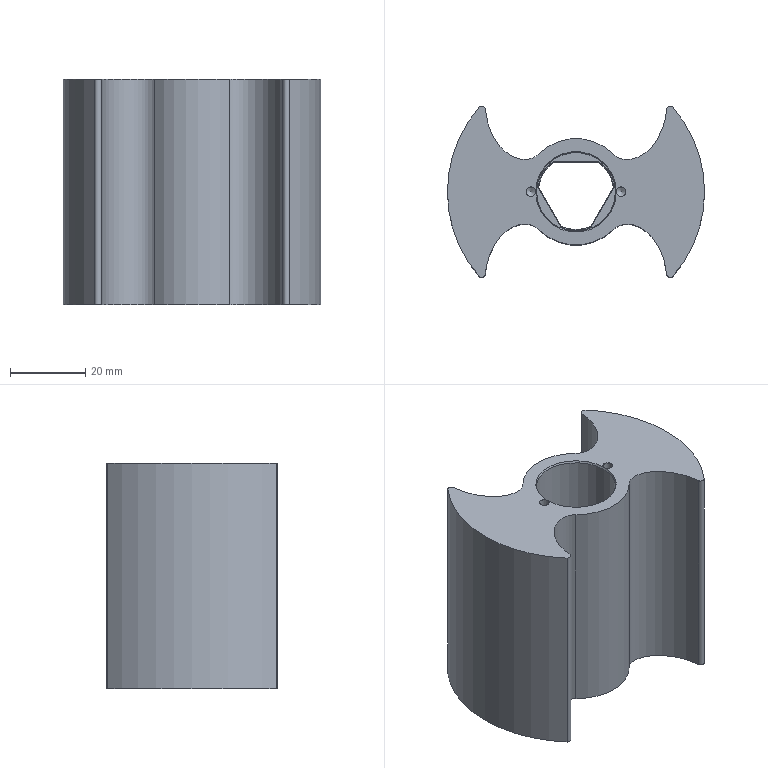NC program | NX | posted with a generic post | part box 68.489 x 45.577 x 60 mm
Lines 1 to 915 of 7016:
N10 G17 G21 G94 G90
(ZLEVEL_PROFILE_COPY_2 , TOOL : D25R0.5)
N12 T05 M6
N14 G54
N16 G17 G0 G90 X47.764 Y-35.886 S2000 M3
N18 G43 Z30. H5
N20 Z-0.349
N22 G94 G1 X43.686 Y-35.094 F1000.
N24 G3 X41.323 Y-35.908 R2.5
N26 G2 X7.37 Y-33.859 R21.45 F2200.
N28 G1 X7.248 Y-33.886
N30 G2 X-7.37 Y-33.859 R34.651
N32 X-41.323 Y-35.908 R21.45
N34 G3 X-43.686 Y-35.094 R2.5
N36 G1 X-47.764 Y-35.886
N38 G0 Z30.
N40 X47.766
N42 Z-0.698
N44 G1 X43.687 Y-35.094 F1000.
N46 G3 X41.323 Y-35.908 R2.5
N48 G2 X7.367 Y-33.86 R21.45 F2200.
N50 G1 X7.248 Y-33.889
N52 G2 X-7.248 Y-33.889 R34.655
N54 G1 X-7.367 Y-33.86
N56 G2 X-41.323 Y-35.908 R21.45
N58 G3 X-43.687 Y-35.094 R2.5
N60 G1 X-47.766 Y-35.886
N62 G0 Z30.
N64 X47.766
N66 Z-1.047
N68 G1 X43.687 Y-35.094 F1000.
N70 G3 X41.323 Y-35.908 R2.5
N72 G2 X7.367 Y-33.86 R21.45 F2200.
N74 G1 X7.248 Y-33.889
N76 G2 X-7.248 Y-33.889 R34.655
N78 G1 X-7.367 Y-33.86
N80 G2 X-41.323 Y-35.908 R21.45
N82 G3 X-43.687 Y-35.094 R2.5
N84 G1 X-47.766 Y-35.886
N86 G0 Z30.
N88 X47.766
N90 Z-1.395
N92 G1 X43.687 Y-35.094 F1000.
N94 G3 X41.323 Y-35.908 R2.5
N96 G2 X7.367 Y-33.86 R21.45 F2200.
N98 G1 X7.248 Y-33.889
N100 G2 X-7.248 Y-33.889 R34.655
N102 G1 X-7.367 Y-33.86
N104 G2 X-41.323 Y-35.908 R21.45
N106 G3 X-43.687 Y-35.094 R2.5
N108 G1 X-47.766 Y-35.886
N110 G0 Z30.
N112 X47.766
N114 Z-1.744
N116 G1 X43.687 Y-35.094 F1000.
N118 G3 X41.323 Y-35.908 R2.5
N120 G2 X7.367 Y-33.86 R21.45 F2200.
N122 G1 X7.248 Y-33.889
N124 G2 X-7.248 Y-33.889 R34.655
N126 G1 X-7.367 Y-33.86
N128 G2 X-41.323 Y-35.908 R21.45
N130 G3 X-43.687 Y-35.094 R2.5
N132 G1 X-47.766 Y-35.886
N134 G0 Z30.
N136 X47.766
N138 Z-2.093
N140 G1 X43.687 Y-35.094 F1000.
N142 G3 X41.323 Y-35.908 R2.5
N144 G2 X7.367 Y-33.86 R21.45 F2200.
N146 G1 X7.248 Y-33.889
N148 G2 X-7.248 Y-33.889 R34.655
N150 G1 X-7.367 Y-33.86
N152 G2 X-41.323 Y-35.908 R21.45
N154 G3 X-43.687 Y-35.094 R2.5
N156 G1 X-47.766 Y-35.886
N158 G0 Z30.
N160 X47.766
N162 Z-2.442
N164 G1 X43.687 Y-35.094 F1000.
N166 G3 X41.323 Y-35.908 R2.5
N168 G2 X7.367 Y-33.86 R21.45 F2200.
N170 G1 X7.248 Y-33.889
N172 G2 X-7.248 Y-33.889 R34.655
N174 G1 X-7.367 Y-33.86
N176 G2 X-41.323 Y-35.908 R21.45
N178 G3 X-43.687 Y-35.094 R2.5
N180 G1 X-47.766 Y-35.886
N182 G0 Z30.
N184 X47.766
N186 Z-2.791
N188 G1 X43.687 Y-35.094 F1000.
N190 G3 X41.323 Y-35.908 R2.5
N192 G2 X7.367 Y-33.86 R21.45 F2200.
N194 G1 X7.248 Y-33.889
N196 G2 X-7.248 Y-33.889 R34.655
N198 G1 X-7.367 Y-33.86
N200 G2 X-41.323 Y-35.908 R21.45
N202 G3 X-43.687 Y-35.094 R2.5
N204 G1 X-47.766 Y-35.886
N206 G0 Z30.
N208 X47.766
N210 Z-3.14
N212 G1 X43.687 Y-35.094 F1000.
N214 G3 X41.323 Y-35.908 R2.5
N216 G2 X7.367 Y-33.86 R21.45 F2200.
N218 G1 X7.248 Y-33.889
N220 G2 X-7.248 Y-33.889 R34.655
N222 G1 X-7.367 Y-33.86
N224 G2 X-41.323 Y-35.908 R21.45
N226 G3 X-43.687 Y-35.094 R2.5
N228 G1 X-47.766 Y-35.886
N230 G0 Z30.
N232 X47.766
N234 Z-3.488
N236 G1 X43.687 Y-35.094 F1000.
N238 G3 X41.323 Y-35.908 R2.5
N240 G2 X7.367 Y-33.86 R21.45 F2200.
N242 G1 X7.248 Y-33.889
N244 G2 X-7.248 Y-33.889 R34.655
N246 G1 X-7.367 Y-33.86
N248 G2 X-41.323 Y-35.908 R21.45
N250 G3 X-43.687 Y-35.094 R2.5
N252 G1 X-47.766 Y-35.886
N254 G0 Z30.
N256 X47.766
N258 Z-3.837
N260 G1 X43.687 Y-35.094 F1000.
N262 G3 X41.323 Y-35.908 R2.5
N264 G2 X7.367 Y-33.86 R21.45 F2200.
N266 G1 X7.248 Y-33.889
N268 G2 X-7.248 Y-33.889 R34.655
N270 G1 X-7.367 Y-33.86
N272 G2 X-41.323 Y-35.908 R21.45
N274 G3 X-43.687 Y-35.094 R2.5
N276 G1 X-47.766 Y-35.886
N278 G0 Z30.
N280 X47.766
N282 Z-4.186
N284 G1 X43.687 Y-35.094 F1000.
N286 G3 X41.323 Y-35.908 R2.5
N288 G2 X7.367 Y-33.86 R21.45 F2200.
N290 G1 X7.248 Y-33.889
N292 G2 X-7.248 Y-33.889 R34.655
N294 G1 X-7.367 Y-33.86
N296 G2 X-41.323 Y-35.908 R21.45
N298 G3 X-43.687 Y-35.094 R2.5
N300 G1 X-47.766 Y-35.886
N302 G0 Z30.
N304 X47.766
N306 Z-4.535
N308 G1 X43.687 Y-35.094 F1000.
N310 G3 X41.323 Y-35.908 R2.5
N312 G2 X7.367 Y-33.86 R21.45 F2200.
N314 G1 X7.248 Y-33.889
N316 G2 X-7.248 Y-33.889 R34.655
N318 G1 X-7.367 Y-33.86
N320 G2 X-41.323 Y-35.908 R21.45
N322 G3 X-43.687 Y-35.094 R2.5
N324 G1 X-47.766 Y-35.886
N326 G0 Z30.
N328 X47.766
N330 Z-4.884
N332 G1 X43.687 Y-35.094 F1000.
N334 G3 X41.323 Y-35.908 R2.5
N336 G2 X7.367 Y-33.86 R21.45 F2200.
N338 G1 X7.248 Y-33.889
N340 G2 X-7.248 Y-33.889 R34.655
N342 G1 X-7.367 Y-33.86
N344 G2 X-41.323 Y-35.908 R21.45
N346 G3 X-43.687 Y-35.094 R2.5
N348 G1 X-47.766 Y-35.886
N350 G0 Z30.
N352 X47.766
N354 Z-5.233
N356 G1 X43.687 Y-35.094 F1000.
N358 G3 X41.323 Y-35.908 R2.5
N360 G2 X7.367 Y-33.86 R21.45 F2200.
N362 G1 X7.248 Y-33.889
N364 G2 X-7.248 Y-33.889 R34.655
N366 G1 X-7.367 Y-33.86
N368 G2 X-41.323 Y-35.908 R21.45
N370 G3 X-43.687 Y-35.094 R2.5
N372 G1 X-47.766 Y-35.886
N374 G0 Z30.
N376 X47.766
N378 Z-5.581
N380 G1 X43.687 Y-35.094 F1000.
N382 G3 X41.323 Y-35.908 R2.5
N384 G2 X7.367 Y-33.86 R21.45 F2200.
N386 G1 X7.248 Y-33.889
N388 G2 X-7.248 Y-33.889 R34.655
N390 G1 X-7.367 Y-33.86
N392 G2 X-41.323 Y-35.908 R21.45
N394 G3 X-43.687 Y-35.094 R2.5
N396 G1 X-47.766 Y-35.886
N398 G0 Z30.
N400 X47.766
N402 Z-5.93
N404 G1 X43.687 Y-35.094 F1000.
N406 G3 X41.323 Y-35.908 R2.5
N408 G2 X7.367 Y-33.86 R21.45 F2200.
N410 G1 X7.248 Y-33.889
N412 G2 X-7.248 Y-33.889 R34.655
N414 G1 X-7.367 Y-33.86
N416 G2 X-41.323 Y-35.908 R21.45
N418 G3 X-43.687 Y-35.094 R2.5
N420 G1 X-47.766 Y-35.886
N422 G0 Z30.
N424 X47.766
N426 Z-6.279
N428 G1 X43.687 Y-35.094 F1000.
N430 G3 X41.323 Y-35.908 R2.5
N432 G2 X7.367 Y-33.86 R21.45 F2200.
N434 G1 X7.248 Y-33.889
N436 G2 X-7.248 Y-33.889 R34.655
N438 G1 X-7.367 Y-33.86
N440 G2 X-41.323 Y-35.908 R21.45
N442 G3 X-43.687 Y-35.094 R2.5
N444 G1 X-47.766 Y-35.886
N446 G0 Z30.
N448 X47.766
N450 Z-6.628
N452 G1 X43.687 Y-35.094 F1000.
N454 G3 X41.323 Y-35.908 R2.5
N456 G2 X7.367 Y-33.86 R21.45 F2200.
N458 G1 X7.248 Y-33.889
N460 G2 X-7.248 Y-33.889 R34.655
N462 G1 X-7.367 Y-33.86
N464 G2 X-41.323 Y-35.908 R21.45
N466 G3 X-43.687 Y-35.094 R2.5
N468 G1 X-47.766 Y-35.886
N470 G0 Z30.
N472 X47.766
N474 Z-6.977
N476 G1 X43.687 Y-35.094 F1000.
N478 G3 X41.323 Y-35.908 R2.5
N480 G2 X7.367 Y-33.86 R21.45 F2200.
N482 G1 X7.248 Y-33.889
N484 G2 X-7.248 Y-33.889 R34.655
N486 G1 X-7.367 Y-33.86
N488 G2 X-41.323 Y-35.908 R21.45
N490 G3 X-43.687 Y-35.094 R2.5
N492 G1 X-47.766 Y-35.886
N494 G0 Z30.
N496 X47.766
N498 Z-7.326
N500 G1 X43.687 Y-35.094 F1000.
N502 G3 X41.323 Y-35.908 R2.5
N504 G2 X7.367 Y-33.86 R21.45 F2200.
N506 G1 X7.248 Y-33.889
N508 G2 X-7.248 Y-33.889 R34.655
N510 G1 X-7.367 Y-33.86
N512 G2 X-41.323 Y-35.908 R21.45
N514 G3 X-43.687 Y-35.094 R2.5
N516 G1 X-47.766 Y-35.886
N518 G0 Z30.
N520 X47.766
N522 Z-7.674
N524 G1 X43.687 Y-35.094 F1000.
N526 G3 X41.323 Y-35.908 R2.5
N528 G2 X7.367 Y-33.86 R21.45 F2200.
N530 G1 X7.248 Y-33.889
N532 G2 X-7.248 Y-33.889 R34.655
N534 G1 X-7.367 Y-33.86
N536 G2 X-41.323 Y-35.908 R21.45
N538 G3 X-43.687 Y-35.094 R2.5
N540 G1 X-47.766 Y-35.886
N542 G0 Z30.
N544 X47.766
N546 Z-8.023
N548 G1 X43.687 Y-35.094 F1000.
N550 G3 X41.323 Y-35.908 R2.5
N552 G2 X7.367 Y-33.86 R21.45 F2200.
N554 G1 X7.248 Y-33.889
N556 G2 X-7.248 Y-33.889 R34.655
N558 G1 X-7.367 Y-33.86
N560 G2 X-41.323 Y-35.908 R21.45
N562 G3 X-43.687 Y-35.094 R2.5
N564 G1 X-47.766 Y-35.886
N566 G0 Z30.
N568 X47.766
N570 Z-8.372
N572 G1 X43.687 Y-35.094 F1000.
N574 G3 X41.323 Y-35.908 R2.5
N576 G2 X7.367 Y-33.86 R21.45 F2200.
N578 G1 X7.248 Y-33.889
N580 G2 X-7.248 Y-33.889 R34.655
N582 G1 X-7.367 Y-33.86
N584 G2 X-41.323 Y-35.908 R21.45
N586 G3 X-43.687 Y-35.094 R2.5
N588 G1 X-47.766 Y-35.886
N590 G0 Z30.
N592 X47.766
N594 Z-8.721
N596 G1 X43.687 Y-35.094 F1000.
N598 G3 X41.323 Y-35.908 R2.5
N600 G2 X7.367 Y-33.86 R21.45 F2200.
N602 G1 X7.248 Y-33.889
N604 G2 X-7.248 Y-33.889 R34.655
N606 G1 X-7.367 Y-33.86
N608 G2 X-41.323 Y-35.908 R21.45
N610 G3 X-43.687 Y-35.094 R2.5
N612 G1 X-47.766 Y-35.886
N614 G0 Z30.
N616 X47.766
N618 Z-9.07
N620 G1 X43.687 Y-35.094 F1000.
N622 G3 X41.323 Y-35.908 R2.5
N624 G2 X7.367 Y-33.86 R21.45 F2200.
N626 G1 X7.248 Y-33.889
N628 G2 X-7.248 Y-33.889 R34.655
N630 G1 X-7.367 Y-33.86
N632 G2 X-41.323 Y-35.908 R21.45
N634 G3 X-43.687 Y-35.094 R2.5
N636 G1 X-47.766 Y-35.886
N638 G0 Z30.
N640 X47.766
N642 Z-9.419
N644 G1 X43.687 Y-35.094 F1000.
N646 G3 X41.323 Y-35.908 R2.5
N648 G2 X7.367 Y-33.86 R21.45 F2200.
N650 G1 X7.248 Y-33.889
N652 G2 X-7.248 Y-33.889 R34.655
N654 G1 X-7.367 Y-33.86
N656 G2 X-41.323 Y-35.908 R21.45
N658 G3 X-43.687 Y-35.094 R2.5
N660 G1 X-47.766 Y-35.886
N662 G0 Z30.
N664 X47.766
N666 Z-9.767
N668 G1 X43.687 Y-35.094 F1000.
N670 G3 X41.323 Y-35.908 R2.5
N672 G2 X7.367 Y-33.86 R21.45 F2200.
N674 G1 X7.248 Y-33.889
N676 G2 X-7.248 Y-33.889 R34.655
N678 G1 X-7.367 Y-33.86
N680 G2 X-41.323 Y-35.908 R21.45
N682 G3 X-43.687 Y-35.094 R2.5
N684 G1 X-47.766 Y-35.886
N686 G0 Z30.
N688 X47.766
N690 Z-10.116
N692 G1 X43.687 Y-35.094 F1000.
N694 G3 X41.323 Y-35.908 R2.5
N696 G2 X7.367 Y-33.86 R21.45 F2200.
N698 G1 X7.248 Y-33.889
N700 G2 X-7.248 Y-33.889 R34.655
N702 G1 X-7.367 Y-33.86
N704 G2 X-41.323 Y-35.908 R21.45
N706 G3 X-43.687 Y-35.094 R2.5
N708 G1 X-47.766 Y-35.886
N710 G0 Z30.
N712 X47.766
N714 Z-10.465
N716 G1 X43.687 Y-35.094 F1000.
N718 G3 X41.323 Y-35.908 R2.5
N720 G2 X7.367 Y-33.86 R21.45 F2200.
N722 G1 X7.248 Y-33.889
N724 G2 X-7.248 Y-33.889 R34.655
N726 G1 X-7.367 Y-33.86
N728 G2 X-41.323 Y-35.908 R21.45
N730 G3 X-43.687 Y-35.094 R2.5
N732 G1 X-47.766 Y-35.886
N734 G0 Z30.
N736 X47.766
N738 Z-10.814
N740 G1 X43.687 Y-35.094 F1000.
N742 G3 X41.323 Y-35.908 R2.5
N744 G2 X7.367 Y-33.86 R21.45 F2200.
N746 G1 X7.248 Y-33.889
N748 G2 X-7.248 Y-33.889 R34.655
N750 G1 X-7.367 Y-33.86
N752 G2 X-41.323 Y-35.908 R21.45
N754 G3 X-43.687 Y-35.094 R2.5
N756 G1 X-47.766 Y-35.886
N758 G0 Z30.
N760 X47.766
N762 Z-11.163
N764 G1 X43.687 Y-35.094 F1000.
N766 G3 X41.323 Y-35.908 R2.5
N768 G2 X7.367 Y-33.86 R21.45 F2200.
N770 G1 X7.248 Y-33.889
N772 G2 X-7.248 Y-33.889 R34.655
N774 G1 X-7.367 Y-33.86
N776 G2 X-41.323 Y-35.908 R21.45
N778 G3 X-43.687 Y-35.094 R2.5
N780 G1 X-47.766 Y-35.886
N782 G0 Z30.
N784 X47.766
N786 Z-11.512
N788 G1 X43.687 Y-35.094 F1000.
N790 G3 X41.323 Y-35.908 R2.5
N792 G2 X7.367 Y-33.86 R21.45 F2200.
N794 G1 X7.248 Y-33.889
N796 G2 X-7.248 Y-33.889 R34.655
N798 G1 X-7.367 Y-33.86
N800 G2 X-41.323 Y-35.908 R21.45
N802 G3 X-43.687 Y-35.094 R2.5
N804 G1 X-47.766 Y-35.886
N806 G0 Z30.
N808 X47.766
N810 Z-11.86
N812 G1 X43.687 Y-35.094 F1000.
N814 G3 X41.323 Y-35.908 R2.5
N816 G2 X7.367 Y-33.86 R21.45 F2200.
N818 G1 X7.248 Y-33.889
N820 G2 X-7.248 Y-33.889 R34.655
N822 G1 X-7.367 Y-33.86
N824 G2 X-41.323 Y-35.908 R21.45
N826 G3 X-43.687 Y-35.094 R2.5
N828 G1 X-47.766 Y-35.886
N830 G0 Z30.
N832 X47.766
N834 Z-12.209
N836 G1 X43.687 Y-35.094 F1000.
N838 G3 X41.323 Y-35.908 R2.5
N840 G2 X7.367 Y-33.86 R21.45 F2200.
N842 G1 X7.248 Y-33.889
N844 G2 X-7.248 Y-33.889 R34.655
N846 G1 X-7.367 Y-33.86
N848 G2 X-41.323 Y-35.908 R21.45
N850 G3 X-43.687 Y-35.094 R2.5
N852 G1 X-47.766 Y-35.886
N854 G0 Z30.
N856 X47.766
N858 Z-12.558
N860 G1 X43.687 Y-35.094 F1000.
N862 G3 X41.323 Y-35.908 R2.5
N864 G2 X7.367 Y-33.86 R21.45 F2200.
N866 G1 X7.248 Y-33.889
N868 G2 X-7.248 Y-33.889 R34.655
N870 G1 X-7.367 Y-33.86
N872 G2 X-41.323 Y-35.908 R21.45
N874 G3 X-43.687 Y-35.094 R2.5
N876 G1 X-47.766 Y-35.886
N878 G0 Z30.
N880 X47.766
N882 Z-12.907
N884 G1 X43.687 Y-35.094 F1000.
N886 G3 X41.323 Y-35.908 R2.5
N888 G2 X7.367 Y-33.86 R21.45 F2200.
N890 G1 X7.248 Y-33.889
N892 G2 X-7.248 Y-33.889 R34.655
N894 G1 X-7.367 Y-33.86
N896 G2 X-41.323 Y-35.908 R21.45
N898 G3 X-43.687 Y-35.094 R2.5
N900 G1 X-47.766 Y-35.886
N902 G0 Z30.
N904 X47.766
N906 Z-13.256
N908 G1 X43.687 Y-35.094 F1000.
N910 G3 X41.323 Y-35.908 R2.5
N912 G2 X7.367 Y-33.86 R21.45 F2200.
N914 G1 X7.248 Y-33.889
N916 G2 X-7.248 Y-33.889 R34.655
N918 G1 X-7.367 Y-33.86
N920 G2 X-41.323 Y-35.908 R21.45
N922 G3 X-43.687 Y-35.094 R2.5
N924 G1 X-47.766 Y-35.886
N926 G0 Z30.
N928 X47.766
N930 Z-13.605
N932 G1 X43.687 Y-35.094 F1000.
N934 G3 X41.323 Y-35.908 R2.5
N936 G2 X7.367 Y-33.86 R21.45 F2200.
N938 G1 X7.248 Y-33.889
N940 G2 X-7.248 Y-33.889 R34.655
N942 G1 X-7.367 Y-33.86
N944 G2 X-41.323 Y-35.908 R21.45
N946 G3 X-43.687 Y-35.094 R2.5
N948 G1 X-47.766 Y-35.886
N950 G0 Z30.
N952 X47.766
N954 Z-13.953
N956 G1 X43.687 Y-35.094 F1000.
N958 G3 X41.323 Y-35.908 R2.5
N960 G2 X7.367 Y-33.86 R21.45 F2200.
N962 G1 X7.248 Y-33.889
N964 G2 X-7.248 Y-33.889 R34.655
N966 G1 X-7.367 Y-33.86
N968 G2 X-41.323 Y-35.908 R21.45
N970 G3 X-43.687 Y-35.094 R2.5
N972 G1 X-47.766 Y-35.886
N974 G0 Z30.
N976 X47.766
N978 Z-14.302
N980 G1 X43.687 Y-35.094 F1000.
N982 G3 X41.323 Y-35.908 R2.5
N984 G2 X7.367 Y-33.86 R21.45 F2200.
N986 G1 X7.248 Y-33.889
N988 G2 X-7.248 Y-33.889 R34.655
N990 G1 X-7.367 Y-33.86
N992 G2 X-41.323 Y-35.908 R21.45
N994 G3 X-43.687 Y-35.094 R2.5
N996 G1 X-47.766 Y-35.886
N998 G0 Z30.
N1000 X47.766
N1002 Z-14.651
N1004 G1 X43.687 Y-35.094 F1000.
N1006 G3 X41.323 Y-35.908 R2.5
N1008 G2 X7.367 Y-33.86 R21.45 F2200.
N1010 G1 X7.248 Y-33.889
N1012 G2 X-7.248 Y-33.889 R34.655
N1014 G1 X-7.367 Y-33.86
N1016 G2 X-41.323 Y-35.908 R21.45
N1018 G3 X-43.687 Y-35.094 R2.5
N1020 G1 X-47.766 Y-35.886
N1022 G0 Z30.
N1024 X47.766
N1026 Z-15.
N1028 G1 X43.687 Y-35.094 F1000.
N1030 G3 X41.323 Y-35.908 R2.5
N1032 G2 X7.367 Y-33.86 R21.45 F2200.
N1034 G1 X7.248 Y-33.889
N1036 G2 X-7.248 Y-33.889 R34.655
N1038 G1 X-7.367 Y-33.86
N1040 G2 X-41.323 Y-35.908 R21.45
N1042 G3 X-43.687 Y-35.094 R2.5
N1044 G1 X-47.766 Y-35.886
N1046 G0 Z30.
N1048 X47.766
N1050 Z-15.349
N1052 G1 X43.687 Y-35.094 F1000.
N1054 G3 X41.323 Y-35.908 R2.5
N1056 G2 X7.367 Y-33.86 R21.45 F2200.
N1058 G1 X7.248 Y-33.889
N1060 G2 X-7.248 Y-33.889 R34.655
N1062 G1 X-7.367 Y-33.86
N1064 G2 X-41.323 Y-35.908 R21.45
N1066 G3 X-43.687 Y-35.094 R2.5
N1068 G1 X-47.766 Y-35.886
N1070 G0 Z30.
N1072 X47.766
N1074 Z-15.698
N1076 G1 X43.687 Y-35.094 F1000.
N1078 G3 X41.323 Y-35.908 R2.5
N1080 G2 X7.367 Y-33.86 R21.45 F2200.
N1082 G1 X7.248 Y-33.889
N1084 G2 X-7.248 Y-33.889 R34.655
N1086 G1 X-7.367 Y-33.86
N1088 G2 X-41.323 Y-35.908 R21.45
N1090 G3 X-43.687 Y-35.094 R2.5
N1092 G1 X-47.766 Y-35.886
N1094 G0 Z30.
N1096 X47.766
N1098 Z-16.047
N1100 G1 X43.687 Y-35.094 F1000.
N1102 G3 X41.323 Y-35.908 R2.5
N1104 G2 X7.367 Y-33.86 R21.45 F2200.
N1106 G1 X7.248 Y-33.889
N1108 G2 X-7.248 Y-33.889 R34.655
N1110 G1 X-7.367 Y-33.86
N1112 G2 X-41.323 Y-35.908 R21.45
N1114 G3 X-43.687 Y-35.094 R2.5
N1116 G1 X-47.766 Y-35.886
N1118 G0 Z30.
N1120 X47.766
N1122 Z-16.395
N1124 G1 X43.687 Y-35.094 F1000.
N1126 G3 X41.323 Y-35.908 R2.5
N1128 G2 X7.367 Y-33.86 R21.45 F2200.
N1130 G1 X7.248 Y-33.889
N1132 G2 X-7.248 Y-33.889 R34.655
N1134 G1 X-7.367 Y-33.86
N1136 G2 X-41.323 Y-35.908 R21.45
N1138 G3 X-43.687 Y-35.094 R2.5
N1140 G1 X-47.766 Y-35.886
N1142 G0 Z30.
N1144 X47.766
N1146 Z-16.744
N1148 G1 X43.687 Y-35.094 F1000.
N1150 G3 X41.323 Y-35.908 R2.5
N1152 G2 X7.367 Y-33.86 R21.45 F2200.
N1154 G1 X7.248 Y-33.889
N1156 G2 X-7.248 Y-33.889 R34.655
N1158 G1 X-7.367 Y-33.86
N1160 G2 X-41.323 Y-35.908 R21.45
N1162 G3 X-43.687 Y-35.094 R2.5
N1164 G1 X-47.766 Y-35.886
N1166 G0 Z30.
N1168 X47.766
N1170 Z-17.093
N1172 G1 X43.687 Y-35.094 F1000.
N1174 G3 X41.323 Y-35.908 R2.5
N1176 G2 X7.367 Y-33.86 R21.45 F2200.
N1178 G1 X7.248 Y-33.889
N1180 G2 X-7.248 Y-33.889 R34.655
N1182 G1 X-7.367 Y-33.86
N1184 G2 X-41.323 Y-35.908 R21.45
N1186 G3 X-43.687 Y-35.094 R2.5
N1188 G1 X-47.766 Y-35.886
N1190 G0 Z30.
N1192 X47.766
N1194 Z-17.442
N1196 G1 X43.687 Y-35.094 F1000.
N1198 G3 X41.323 Y-35.908 R2.5
N1200 G2 X7.367 Y-33.86 R21.45 F2200.
N1202 G1 X7.248 Y-33.889
N1204 G2 X-7.248 Y-33.889 R34.655
N1206 G1 X-7.367 Y-33.86
N1208 G2 X-41.323 Y-35.908 R21.45
N1210 G3 X-43.687 Y-35.094 R2.5
N1212 G1 X-47.766 Y-35.886
N1214 G0 Z30.
N1216 X47.766
N1218 Z-17.791
N1220 G1 X43.687 Y-35.094 F1000.
N1222 G3 X41.323 Y-35.908 R2.5
N1224 G2 X7.367 Y-33.86 R21.45 F2200.
N1226 G1 X7.248 Y-33.889
N1228 G2 X-7.248 Y-33.889 R34.655
N1230 G1 X-7.367 Y-33.86
N1232 G2 X-41.323 Y-35.908 R21.45
N1234 G3 X-43.687 Y-35.094 R2.5
N1236 G1 X-47.766 Y-35.886
N1238 G0 Z30.
N1240 X47.766
N1242 Z-18.14
N1244 G1 X43.687 Y-35.094 F1000.
N1246 G3 X41.323 Y-35.908 R2.5
N1248 G2 X7.367 Y-33.86 R21.45 F2200.
N1250 G1 X7.248 Y-33.889
N1252 G2 X-7.248 Y-33.889 R34.655
N1254 G1 X-7.367 Y-33.86
N1256 G2 X-41.323 Y-35.908 R21.45
N1258 G3 X-43.687 Y-35.094 R2.5
N1260 G1 X-47.766 Y-35.886
N1262 G0 Z30.
N1264 X47.766
N1266 Z-18.488
N1268 G1 X43.687 Y-35.094 F1000.
N1270 G3 X41.323 Y-35.908 R2.5
N1272 G2 X7.367 Y-33.86 R21.45 F2200.
N1274 G1 X7.248 Y-33.889
N1276 G2 X-7.248 Y-33.889 R34.655
N1278 G1 X-7.367 Y-33.86
N1280 G2 X-41.323 Y-35.908 R21.45
N1282 G3 X-43.687 Y-35.094 R2.5
N1284 G1 X-47.766 Y-35.886
N1286 G0 Z30.
N1288 X47.766
N1290 Z-18.837
N1292 G1 X43.687 Y-35.094 F1000.
N1294 G3 X41.323 Y-35.908 R2.5
N1296 G2 X7.367 Y-33.86 R21.45 F2200.
N1298 G1 X7.248 Y-33.889
N1300 G2 X-7.248 Y-33.889 R34.655
N1302 G1 X-7.367 Y-33.86
N1304 G2 X-41.323 Y-35.908 R21.45
N1306 G3 X-43.687 Y-35.094 R2.5
N1308 G1 X-47.766 Y-35.886
N1310 G0 Z30.
N1312 X47.766
N1314 Z-19.186
N1316 G1 X43.687 Y-35.094 F1000.
N1318 G3 X41.323 Y-35.908 R2.5
N1320 G2 X7.367 Y-33.86 R21.45 F2200.
N1322 G1 X7.248 Y-33.889
N1324 G2 X-7.248 Y-33.889 R34.655
N1326 G1 X-7.367 Y-33.86
N1328 G2 X-41.323 Y-35.908 R21.45
N1330 G3 X-43.687 Y-35.094 R2.5
N1332 G1 X-47.766 Y-35.886
N1334 G0 Z30.
N1336 X47.766
N1338 Z-19.535
N1340 G1 X43.687 Y-35.094 F1000.
N1342 G3 X41.323 Y-35.908 R2.5
N1344 G2 X7.367 Y-33.86 R21.45 F2200.
N1346 G1 X7.248 Y-33.889
N1348 G2 X-7.248 Y-33.889 R34.655
N1350 G1 X-7.367 Y-33.86
N1352 G2 X-41.323 Y-35.908 R21.45
N1354 G3 X-43.687 Y-35.094 R2.5
N1356 G1 X-47.766 Y-35.886
N1358 G0 Z30.
N1360 X47.766
N1362 Z-19.884
N1364 G1 X43.687 Y-35.094 F1000.
N1366 G3 X41.323 Y-35.908 R2.5
N1368 G2 X7.367 Y-33.86 R21.45 F2200.
N1370 G1 X7.248 Y-33.889
N1372 G2 X-7.248 Y-33.889 R34.655
N1374 G1 X-7.367 Y-33.86
N1376 G2 X-41.323 Y-35.908 R21.45
N1378 G3 X-43.687 Y-35.094 R2.5
N1380 G1 X-47.766 Y-35.886
N1382 G0 Z30.
N1384 X47.766
N1386 Z-20.233
N1388 G1 X43.687 Y-35.094 F1000.
N1390 G3 X41.323 Y-35.908 R2.5
N1392 G2 X7.367 Y-33.86 R21.45 F2200.
N1394 G1 X7.248 Y-33.889
N1396 G2 X-7.248 Y-33.889 R34.655
N1398 G1 X-7.367 Y-33.86
N1400 G2 X-41.323 Y-35.908 R21.45
N1402 G3 X-43.687 Y-35.094 R2.5
N1404 G1 X-47.766 Y-35.886
N1406 G0 Z30.
N1408 X47.766
N1410 Z-20.581
N1412 G1 X43.687 Y-35.094 F1000.
N1414 G3 X41.323 Y-35.908 R2.5
N1416 G2 X7.367 Y-33.86 R21.45 F2200.
N1418 G1 X7.248 Y-33.889
N1420 G2 X-7.248 Y-33.889 R34.655
N1422 G1 X-7.367 Y-33.86
N1424 G2 X-41.323 Y-35.908 R21.45
N1426 G3 X-43.687 Y-35.094 R2.5
N1428 G1 X-47.766 Y-35.886
N1430 G0 Z30.
N1432 X47.766
N1434 Z-20.93
N1436 G1 X43.687 Y-35.094 F1000.
N1438 G3 X41.323 Y-35.908 R2.5
N1440 G2 X7.367 Y-33.86 R21.45 F2200.
N1442 G1 X7.248 Y-33.889
N1444 G2 X-7.248 Y-33.889 R34.655
N1446 G1 X-7.367 Y-33.86
N1448 G2 X-41.323 Y-35.908 R21.45
N1450 G3 X-43.687 Y-35.094 R2.5
N1452 G1 X-47.766 Y-35.886
N1454 G0 Z30.
N1456 X47.766
N1458 Z-21.279
N1460 G1 X43.687 Y-35.094 F1000.
N1462 G3 X41.323 Y-35.908 R2.5
N1464 G2 X7.367 Y-33.86 R21.45 F2200.
N1466 G1 X7.248 Y-33.889
N1468 G2 X-7.248 Y-33.889 R34.655
N1470 G1 X-7.367 Y-33.86
N1472 G2 X-41.323 Y-35.908 R21.45
N1474 G3 X-43.687 Y-35.094 R2.5
N1476 G1 X-47.766 Y-35.886
N1478 G0 Z30.
N1480 X47.766
N1482 Z-21.628
N1484 G1 X43.687 Y-35.094 F1000.
N1486 G3 X41.323 Y-35.908 R2.5
N1488 G2 X7.367 Y-33.86 R21.45 F2200.
N1490 G1 X7.248 Y-33.889
N1492 G2 X-7.248 Y-33.889 R34.655
N1494 G1 X-7.367 Y-33.86
N1496 G2 X-41.323 Y-35.908 R21.45
N1498 G3 X-43.687 Y-35.094 R2.5
N1500 G1 X-47.766 Y-35.886
N1502 G0 Z30.
N1504 X47.766
N1506 Z-21.977
N1508 G1 X43.687 Y-35.094 F1000.
N1510 G3 X41.323 Y-35.908 R2.5
N1512 G2 X7.367 Y-33.86 R21.45 F2200.
N1514 G1 X7.248 Y-33.889
N1516 G2 X-7.248 Y-33.889 R34.655
N1518 G1 X-7.367 Y-33.86
N1520 G2 X-41.323 Y-35.908 R21.45
N1522 G3 X-43.687 Y-35.094 R2.5
N1524 G1 X-47.766 Y-35.886
N1526 G0 Z30.
N1528 X47.766
N1530 Z-22.326
N1532 G1 X43.687 Y-35.094 F1000.
N1534 G3 X41.323 Y-35.908 R2.5
N1536 G2 X7.367 Y-33.86 R21.45 F2200.
N1538 G1 X7.248 Y-33.889
N1540 G2 X-7.248 Y-33.889 R34.655
N1542 G1 X-7.367 Y-33.86
N1544 G2 X-41.323 Y-35.908 R21.45
N1546 G3 X-43.687 Y-35.094 R2.5
N1548 G1 X-47.766 Y-35.886
N1550 G0 Z30.
N1552 X47.766
N1554 Z-22.674
N1556 G1 X43.687 Y-35.094 F1000.
N1558 G3 X41.323 Y-35.908 R2.5
N1560 G2 X7.367 Y-33.86 R21.45 F2200.
N1562 G1 X7.248 Y-33.889
N1564 G2 X-7.248 Y-33.889 R34.655
N1566 G1 X-7.367 Y-33.86
N1568 G2 X-41.323 Y-35.908 R21.45
N1570 G3 X-43.687 Y-35.094 R2.5
N1572 G1 X-47.766 Y-35.886
N1574 G0 Z30.
N1576 X47.766
N1578 Z-23.023
N1580 G1 X43.687 Y-35.094 F1000.
N1582 G3 X41.323 Y-35.908 R2.5
N1584 G2 X7.367 Y-33.86 R21.45 F2200.
N1586 G1 X7.248 Y-33.889
N1588 G2 X-7.248 Y-33.889 R34.655
N1590 G1 X-7.367 Y-33.86
N1592 G2 X-41.323 Y-35.908 R21.45
N1594 G3 X-43.687 Y-35.094 R2.5
N1596 G1 X-47.766 Y-35.886
N1598 G0 Z30.
N1600 X47.766
N1602 Z-23.372
N1604 G1 X43.687 Y-35.094 F1000.
N1606 G3 X41.323 Y-35.908 R2.5
N1608 G2 X7.367 Y-33.86 R21.45 F2200.
N1610 G1 X7.248 Y-33.889
N1612 G2 X-7.248 Y-33.889 R34.655
N1614 G1 X-7.367 Y-33.86
N1616 G2 X-41.323 Y-35.908 R21.45
N1618 G3 X-43.687 Y-35.094 R2.5
N1620 G1 X-47.766 Y-35.886
N1622 G0 Z30.
N1624 X47.766
N1626 Z-23.721
N1628 G1 X43.687 Y-35.094 F1000.
N1630 G3 X41.323 Y-35.908 R2.5
N1632 G2 X7.367 Y-33.86 R21.45 F2200.
N1634 G1 X7.248 Y-33.889
N1636 G2 X-7.248 Y-33.889 R34.655
N1638 G1 X-7.367 Y-33.86
N1640 G2 X-41.323 Y-35.908 R21.45
N1642 G3 X-43.687 Y-35.094 R2.5
N1644 G1 X-47.766 Y-35.886
N1646 G0 Z30.
N1648 X47.766
N1650 Z-24.07
N1652 G1 X43.687 Y-35.094 F1000.
N1654 G3 X41.323 Y-35.908 R2.5
N1656 G2 X7.367 Y-33.86 R21.45 F2200.
N1658 G1 X7.248 Y-33.889
N1660 G2 X-7.248 Y-33.889 R34.655
N1662 G1 X-7.367 Y-33.86
N1664 G2 X-41.323 Y-35.908 R21.45
N1666 G3 X-43.687 Y-35.094 R2.5
N1668 G1 X-47.766 Y-35.886
N1670 G0 Z30.
N1672 X47.766
N1674 Z-24.419
N1676 G1 X43.687 Y-35.094 F1000.
N1678 G3 X41.323 Y-35.908 R2.5
N1680 G2 X7.367 Y-33.86 R21.45 F2200.
N1682 G1 X7.248 Y-33.889
N1684 G2 X-7.248 Y-33.889 R34.655
N1686 G1 X-7.367 Y-33.86
N1688 G2 X-41.323 Y-35.908 R21.45
N1690 G3 X-43.687 Y-35.094 R2.5
N1692 G1 X-47.766 Y-35.886
N1694 G0 Z30.
N1696 X47.766
N1698 Z-24.767
N1700 G1 X43.687 Y-35.094 F1000.
N1702 G3 X41.323 Y-35.908 R2.5
N1704 G2 X7.367 Y-33.86 R21.45 F2200.
N1706 G1 X7.248 Y-33.889
N1708 G2 X-7.248 Y-33.889 R34.655
N1710 G1 X-7.367 Y-33.86
N1712 G2 X-41.323 Y-35.908 R21.45
N1714 G3 X-43.687 Y-35.094 R2.5
N1716 G1 X-47.766 Y-35.886
N1718 G0 Z30.
N1720 X47.766
N1722 Z-25.116
N1724 G1 X43.687 Y-35.094 F1000.
N1726 G3 X41.323 Y-35.908 R2.5
N1728 G2 X7.367 Y-33.86 R21.45 F2200.
N1730 G1 X7.248 Y-33.889
N1732 G2 X-7.248 Y-33.889 R34.655
N1734 G1 X-7.367 Y-33.86
N1736 G2 X-41.323 Y-35.908 R21.45
N1738 G3 X-43.687 Y-35.094 R2.5
N1740 G1 X-47.766 Y-35.886
N1742 G0 Z30.
N1744 X47.766
N1746 Z-25.465
N1748 G1 X43.687 Y-35.094 F1000.
N1750 G3 X41.323 Y-35.908 R2.5
N1752 G2 X7.367 Y-33.86 R21.45 F2200.
N1754 G1 X7.248 Y-33.889
N1756 G2 X-7.248 Y-33.889 R34.655
N1758 G1 X-7.367 Y-33.86
N1760 G2 X-41.323 Y-35.908 R21.45
N1762 G3 X-43.687 Y-35.094 R2.5
N1764 G1 X-47.766 Y-35.886
N1766 G0 Z30.
N1768 X47.766
N1770 Z-25.814
N1772 G1 X43.687 Y-35.094 F1000.
N1774 G3 X41.323 Y-35.908 R2.5
N1776 G2 X7.367 Y-33.86 R21.45 F2200.
N1778 G1 X7.248 Y-33.889
N1780 G2 X-7.248 Y-33.889 R34.655
N1782 G1 X-7.367 Y-33.86
N1784 G2 X-41.323 Y-35.908 R21.45
N1786 G3 X-43.687 Y-35.094 R2.5
N1788 G1 X-47.766 Y-35.886
N1790 G0 Z30.
N1792 X47.766
N1794 Z-26.163
N1796 G1 X43.687 Y-35.094 F1000.
N1798 G3 X41.323 Y-35.908 R2.5
N1800 G2 X7.367 Y-33.86 R21.45 F2200.
N1802 G1 X7.248 Y-33.889
N1804 G2 X-7.248 Y-33.889 R34.655
N1806 G1 X-7.367 Y-33.86
N1808 G2 X-41.323 Y-35.908 R21.45
N1810 G3 X-43.687 Y-35.094 R2.5
N1812 G1 X-47.766 Y-35.886
N1814 G0 Z30.
N1816 X47.766
N1818 Z-26.512
N1820 G1 X43.687 Y-35.094 F1000.
N1822 G3 X41.323 Y-35.908 R2.5
N1824 G2 X7.367 Y-33.86 R21.45 F2200.
N1826 G1 X7.248 Y-33.889
N1828 G2 X-7.248 Y-33.889 R34.655